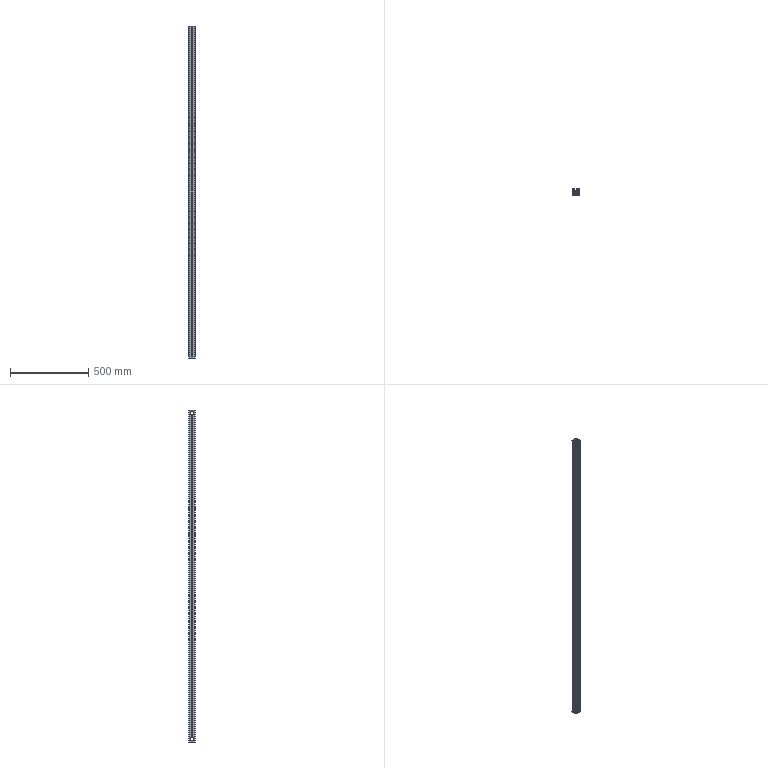Part | SolidWorks | features BaseBody 1, HoleWzd 1, MoveFace 1 | 1 solid | 242 faces | box 40 x 40 x 2120 mm | volume 1246811 mm3 | plane 187 | cylinder 55 | commonest cylinder face diameters 6.8 x15 2 x14 19 x12 1 x6 5 x4 9 x4